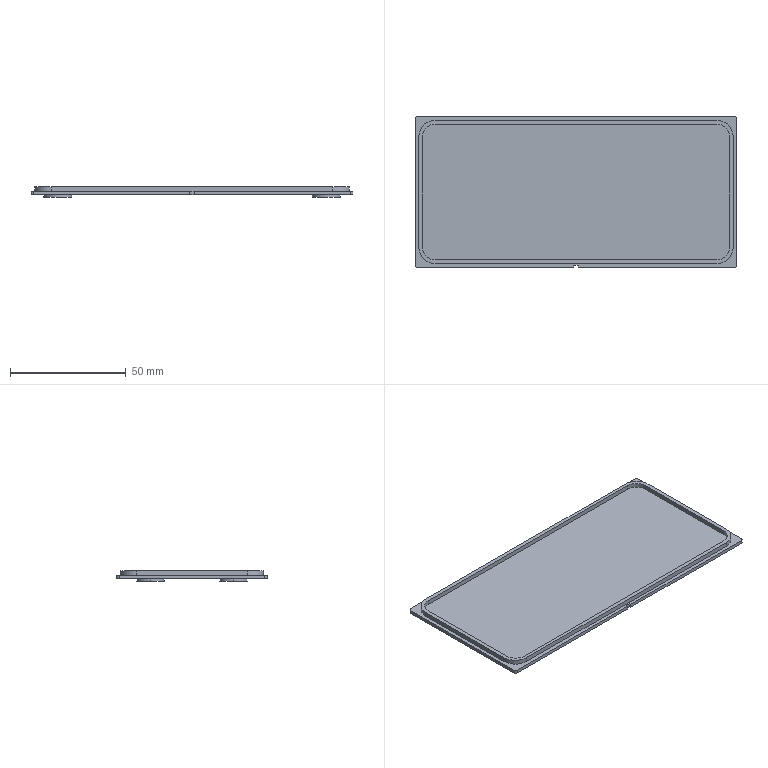Part | SolidWorks | features ICE 4, Extrusion 1 | 1 solid | 56 faces | box 139 x 65 x 4.5 mm | volume 14558 mm3 | cylinder 28 | plane 28 | commonest cylinder face diameters 10.2 x8 12 x8 2 x4 10.8 x4 14 x4